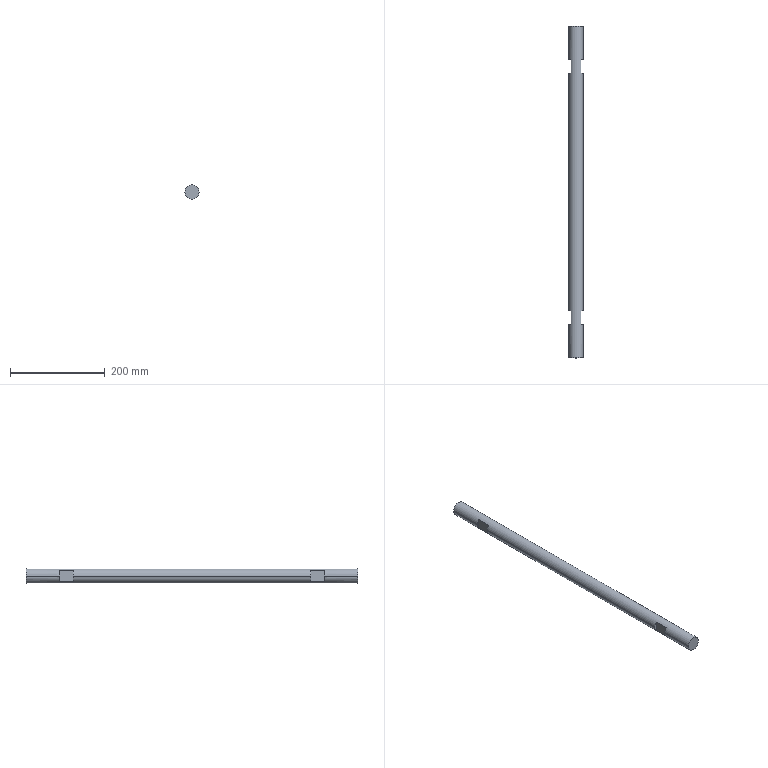Part | NX | features BREP 1 | 1 solid | 16 faces | box 30 x 700 x 30 mm | volume 485508 mm3 | plane 14 | cylinder 2 | commonest cylinder face diameters 30 x2
STEP:
#1=CARTESIAN_POINT('',(15.,-350.,0.));
#2=VERTEX_POINT('',#1);
#3=CARTESIAN_POINT('',(-15.,-350.,0.));
#4=VERTEX_POINT('',#3);
#5=CARTESIAN_POINT('',(0.,-350.,0.));
#6=DIRECTION('',(0.,-1.,0.));
#7=DIRECTION('',(1.,0.,0.));
#8=AXIS2_PLACEMENT_3D('',#5,#6,#7);
#9=CIRCLE('',#8,15.);
#10=EDGE_CURVE('',#2,#4,#9,.T.);
#11=ORIENTED_EDGE('',*,*,#10,.T.);
#12=CARTESIAN_POINT('',(0.,-350.,0.));
#13=DIRECTION('',(0.,-1.,0.));
#14=DIRECTION('',(-1.,0.,0.));
#15=AXIS2_PLACEMENT_3D('',#12,#13,#14);
#16=CIRCLE('',#15,15.);
#17=EDGE_CURVE('',#4,#2,#16,.T.);
#18=ORIENTED_EDGE('',*,*,#17,.T.);
#19=EDGE_LOOP('',(#11,#18));
#20=FACE_BOUND('',#19,.T.);
#21=CARTESIAN_POINT('',(0.,-350.,0.));
#22=DIRECTION('',(0.,1.,0.));
#23=DIRECTION('',(1.,0.,0.));
#24=AXIS2_PLACEMENT_3D('',#21,#22,#23);
#25=PLANE('',#24);
#26=ADVANCED_FACE('',(#20),#25,.F.);
#27=CARTESIAN_POINT('',(10.,-250.,-11.18));
#28=VERTEX_POINT('',#27);
#29=CARTESIAN_POINT('',(15.,-250.,0.));
#30=VERTEX_POINT('',#29);
#31=CARTESIAN_POINT('',(0.,-250.,0.));
#32=DIRECTION('',(0.,-1.,0.));
#33=DIRECTION('',(0.6667,0.,-0.7454));
#34=AXIS2_PLACEMENT_3D('',#31,#32,#33);
#35=CIRCLE('',#34,15.);
#36=EDGE_CURVE('',#28,#30,#35,.T.);
#37=ORIENTED_EDGE('',*,*,#36,.F.);
#38=CARTESIAN_POINT('',(10.,-280.,-11.18));
#39=VERTEX_POINT('',#38);
#40=CARTESIAN_POINT('',(10.,-250.,-11.18));
#41=DIRECTION('',(0.,-1.,0.));
#42=VECTOR('',#41,1000.);
#43=LINE('',#40,#42);
#44=EDGE_CURVE('',#28,#39,#43,.T.);
#45=ORIENTED_EDGE('',*,*,#44,.T.);
#46=CARTESIAN_POINT('',(15.,-280.,0.));
#47=VERTEX_POINT('',#46);
#48=CARTESIAN_POINT('',(0.,-280.,0.));
#49=DIRECTION('',(0.,1.,0.));
#50=DIRECTION('',(1.,0.,0.));
#51=AXIS2_PLACEMENT_3D('',#48,#49,#50);
#52=CIRCLE('',#51,15.);
#53=EDGE_CURVE('',#47,#39,#52,.T.);
#54=ORIENTED_EDGE('',*,*,#53,.F.);
#55=CARTESIAN_POINT('',(15.,-280.,0.));
#56=DIRECTION('',(0.,-1.,0.));
#57=VECTOR('',#56,1000.);
#58=LINE('',#55,#57);
#59=EDGE_CURVE('',#47,#2,#58,.T.);
#60=ORIENTED_EDGE('',*,*,#59,.T.);
#61=ORIENTED_EDGE('',*,*,#17,.F.);
#62=CARTESIAN_POINT('',(-15.,-280.,0.));
#63=VERTEX_POINT('',#62);
#64=CARTESIAN_POINT('',(-15.,-280.,0.));
#65=DIRECTION('',(0.,-1.,0.));
#66=VECTOR('',#65,1000.);
#67=LINE('',#64,#66);
#68=EDGE_CURVE('',#63,#4,#67,.T.);
#69=ORIENTED_EDGE('',*,*,#68,.F.);
#70=CARTESIAN_POINT('',(-10.,-280.,-11.18));
#71=VERTEX_POINT('',#70);
#72=CARTESIAN_POINT('',(0.,-280.,0.));
#73=DIRECTION('',(0.,1.,0.));
#74=DIRECTION('',(-0.6667,0.,-0.7454));
#75=AXIS2_PLACEMENT_3D('',#72,#73,#74);
#76=CIRCLE('',#75,15.);
#77=EDGE_CURVE('',#71,#63,#76,.T.);
#78=ORIENTED_EDGE('',*,*,#77,.F.);
#79=CARTESIAN_POINT('',(-10.,-250.,-11.18));
#80=VERTEX_POINT('',#79);
#81=CARTESIAN_POINT('',(-10.,-280.,-11.18));
#82=DIRECTION('',(0.,1.,0.));
#83=VECTOR('',#82,1000.);
#84=LINE('',#81,#83);
#85=EDGE_CURVE('',#71,#80,#84,.T.);
#86=ORIENTED_EDGE('',*,*,#85,.T.);
#87=CARTESIAN_POINT('',(-15.,-250.,0.));
#88=VERTEX_POINT('',#87);
#89=CARTESIAN_POINT('',(0.,-250.,0.));
#90=DIRECTION('',(0.,-1.,0.));
#91=DIRECTION('',(-1.,0.,0.));
#92=AXIS2_PLACEMENT_3D('',#89,#90,#91);
#93=CIRCLE('',#92,15.);
#94=EDGE_CURVE('',#88,#80,#93,.T.);
#95=ORIENTED_EDGE('',*,*,#94,.F.);
#96=CARTESIAN_POINT('',(-15.,250.,0.));
#97=VERTEX_POINT('',#96);
#98=CARTESIAN_POINT('',(-15.,250.,0.));
#99=DIRECTION('',(0.,-1.,0.));
#100=VECTOR('',#99,1000.);
#101=LINE('',#98,#100);
#102=EDGE_CURVE('',#97,#88,#101,.T.);
#103=ORIENTED_EDGE('',*,*,#102,.F.);
#104=CARTESIAN_POINT('',(-10.,250.,-11.18));
#105=VERTEX_POINT('',#104);
#106=CARTESIAN_POINT('',(0.,250.,0.));
#107=DIRECTION('',(0.,1.,0.));
#108=DIRECTION('',(-0.6667,0.,-0.7454));
#109=AXIS2_PLACEMENT_3D('',#106,#107,#108);
#110=CIRCLE('',#109,15.);
#111=EDGE_CURVE('',#105,#97,#110,.T.);
#112=ORIENTED_EDGE('',*,*,#111,.F.);
#113=CARTESIAN_POINT('',(-10.,280.,-11.18));
#114=VERTEX_POINT('',#113);
#115=CARTESIAN_POINT('',(-10.,250.,-11.18));
#116=DIRECTION('',(0.,1.,0.));
#117=VECTOR('',#116,1000.);
#118=LINE('',#115,#117);
#119=EDGE_CURVE('',#105,#114,#118,.T.);
#120=ORIENTED_EDGE('',*,*,#119,.T.);
#121=CARTESIAN_POINT('',(-15.,280.,0.));
#122=VERTEX_POINT('',#121);
#123=CARTESIAN_POINT('',(0.,280.,0.));
#124=DIRECTION('',(0.,-1.,0.));
#125=DIRECTION('',(-1.,0.,0.));
#126=AXIS2_PLACEMENT_3D('',#123,#124,#125);
#127=CIRCLE('',#126,15.);
#128=EDGE_CURVE('',#122,#114,#127,.T.);
#129=ORIENTED_EDGE('',*,*,#128,.F.);
#130=CARTESIAN_POINT('',(-15.,350.,0.));
#131=VERTEX_POINT('',#130);
#132=CARTESIAN_POINT('',(-15.,350.,0.));
#133=DIRECTION('',(0.,-1.,0.));
#134=VECTOR('',#133,1000.);
#135=LINE('',#132,#134);
#136=EDGE_CURVE('',#122,#131,#135,.F.);
#137=ORIENTED_EDGE('',*,*,#136,.T.);
#138=CARTESIAN_POINT('',(15.,350.,0.));
#139=VERTEX_POINT('',#138);
#140=CARTESIAN_POINT('',(0.,350.,0.));
#141=DIRECTION('',(0.,1.,0.));
#142=DIRECTION('',(1.,0.,0.));
#143=AXIS2_PLACEMENT_3D('',#140,#141,#142);
#144=CIRCLE('',#143,15.);
#145=EDGE_CURVE('',#139,#131,#144,.T.);
#146=ORIENTED_EDGE('',*,*,#145,.F.);
#147=CARTESIAN_POINT('',(15.,280.,0.));
#148=VERTEX_POINT('',#147);
#149=CARTESIAN_POINT('',(15.,350.,0.));
#150=DIRECTION('',(0.,-1.,0.));
#151=VECTOR('',#150,1000.);
#152=LINE('',#149,#151);
#153=EDGE_CURVE('',#148,#139,#152,.F.);
#154=ORIENTED_EDGE('',*,*,#153,.F.);
#155=CARTESIAN_POINT('',(10.,280.,-11.18));
#156=VERTEX_POINT('',#155);
#157=CARTESIAN_POINT('',(0.,280.,0.));
#158=DIRECTION('',(0.,-1.,0.));
#159=DIRECTION('',(0.6667,0.,-0.7454));
#160=AXIS2_PLACEMENT_3D('',#157,#158,#159);
#161=CIRCLE('',#160,15.);
#162=EDGE_CURVE('',#156,#148,#161,.T.);
#163=ORIENTED_EDGE('',*,*,#162,.F.);
#164=CARTESIAN_POINT('',(10.,250.,-11.18));
#165=VERTEX_POINT('',#164);
#166=CARTESIAN_POINT('',(10.,280.,-11.18));
#167=DIRECTION('',(0.,-1.,0.));
#168=VECTOR('',#167,1000.);
#169=LINE('',#166,#168);
#170=EDGE_CURVE('',#156,#165,#169,.T.);
#171=ORIENTED_EDGE('',*,*,#170,.T.);
#172=CARTESIAN_POINT('',(15.,250.,0.));
#173=VERTEX_POINT('',#172);
#174=CARTESIAN_POINT('',(0.,250.,0.));
#175=DIRECTION('',(0.,1.,0.));
#176=DIRECTION('',(1.,0.,0.));
#177=AXIS2_PLACEMENT_3D('',#174,#175,#176);
#178=CIRCLE('',#177,15.);
#179=EDGE_CURVE('',#173,#165,#178,.T.);
#180=ORIENTED_EDGE('',*,*,#179,.F.);
#181=CARTESIAN_POINT('',(15.,250.,0.));
#182=DIRECTION('',(0.,-1.,0.));
#183=VECTOR('',#182,1000.);
#184=LINE('',#181,#183);
#185=EDGE_CURVE('',#173,#30,#184,.T.);
#186=ORIENTED_EDGE('',*,*,#185,.T.);
#187=EDGE_LOOP('',(#37,#45,#54,#60,#61,#69,#78,#86,#95,#103,#112,#120,#129,#137,#146,#154,#163,#171,#180,#186));
#188=FACE_BOUND('',#187,.T.);
#189=CARTESIAN_POINT('',(0.,0.,0.));
#190=DIRECTION('',(0.,1.,0.));
#191=DIRECTION('',(-1.,0.,0.));
#192=AXIS2_PLACEMENT_3D('',#189,#190,#191);
#193=CYLINDRICAL_SURFACE('',#192,15.);
#194=ADVANCED_FACE('',(#188),#193,.T.);
#195=CARTESIAN_POINT('',(-10.,-250.,11.18));
#196=VERTEX_POINT('',#195);
#197=CARTESIAN_POINT('',(0.,-250.,0.));
#198=DIRECTION('',(0.,-1.,0.));
#199=DIRECTION('',(-0.6667,0.,0.7454));
#200=AXIS2_PLACEMENT_3D('',#197,#198,#199);
#201=CIRCLE('',#200,15.);
#202=EDGE_CURVE('',#196,#88,#201,.T.);
#203=ORIENTED_EDGE('',*,*,#202,.F.);
#204=CARTESIAN_POINT('',(-10.,-280.,11.18));
#205=VERTEX_POINT('',#204);
#206=CARTESIAN_POINT('',(-10.,-250.,11.18));
#207=DIRECTION('',(0.,-1.,0.));
#208=VECTOR('',#207,1000.);
#209=LINE('',#206,#208);
#210=EDGE_CURVE('',#196,#205,#209,.T.);
#211=ORIENTED_EDGE('',*,*,#210,.T.);
#212=CARTESIAN_POINT('',(0.,-280.,0.));
#213=DIRECTION('',(0.,1.,0.));
#214=DIRECTION('',(-1.,0.,0.));
#215=AXIS2_PLACEMENT_3D('',#212,#213,#214);
#216=CIRCLE('',#215,15.);
#217=EDGE_CURVE('',#63,#205,#216,.T.);
#218=ORIENTED_EDGE('',*,*,#217,.F.);
#219=ORIENTED_EDGE('',*,*,#68,.T.);
#220=ORIENTED_EDGE('',*,*,#10,.F.);
#221=ORIENTED_EDGE('',*,*,#59,.F.);
#222=CARTESIAN_POINT('',(10.,-280.,11.18));
#223=VERTEX_POINT('',#222);
#224=CARTESIAN_POINT('',(0.,-280.,0.));
#225=DIRECTION('',(0.,1.,0.));
#226=DIRECTION('',(0.6667,0.,0.7454));
#227=AXIS2_PLACEMENT_3D('',#224,#225,#226);
#228=CIRCLE('',#227,15.);
#229=EDGE_CURVE('',#223,#47,#228,.T.);
#230=ORIENTED_EDGE('',*,*,#229,.F.);
#231=CARTESIAN_POINT('',(10.,-250.,11.18));
#232=VERTEX_POINT('',#231);
#233=CARTESIAN_POINT('',(10.,-280.,11.18));
#234=DIRECTION('',(0.,1.,0.));
#235=VECTOR('',#234,1000.);
#236=LINE('',#233,#235);
#237=EDGE_CURVE('',#223,#232,#236,.T.);
#238=ORIENTED_EDGE('',*,*,#237,.T.);
#239=CARTESIAN_POINT('',(0.,-250.,0.));
#240=DIRECTION('',(0.,-1.,0.));
#241=DIRECTION('',(1.,0.,0.));
#242=AXIS2_PLACEMENT_3D('',#239,#240,#241);
#243=CIRCLE('',#242,15.);
#244=EDGE_CURVE('',#30,#232,#243,.T.);
#245=ORIENTED_EDGE('',*,*,#244,.F.);
#246=ORIENTED_EDGE('',*,*,#185,.F.);
#247=CARTESIAN_POINT('',(10.,250.,11.18));
#248=VERTEX_POINT('',#247);
#249=CARTESIAN_POINT('',(0.,250.,0.));
#250=DIRECTION('',(0.,1.,0.));
#251=DIRECTION('',(0.6667,0.,0.7454));
#252=AXIS2_PLACEMENT_3D('',#249,#250,#251);
#253=CIRCLE('',#252,15.);
#254=EDGE_CURVE('',#248,#173,#253,.T.);
#255=ORIENTED_EDGE('',*,*,#254,.F.);
#256=CARTESIAN_POINT('',(10.,280.,11.18));
#257=VERTEX_POINT('',#256);
#258=CARTESIAN_POINT('',(10.,250.,11.18));
#259=DIRECTION('',(0.,1.,0.));
#260=VECTOR('',#259,1000.);
#261=LINE('',#258,#260);
#262=EDGE_CURVE('',#248,#257,#261,.T.);
#263=ORIENTED_EDGE('',*,*,#262,.T.);
#264=CARTESIAN_POINT('',(0.,280.,0.));
#265=DIRECTION('',(0.,-1.,0.));
#266=DIRECTION('',(1.,0.,0.));
#267=AXIS2_PLACEMENT_3D('',#264,#265,#266);
#268=CIRCLE('',#267,15.);
#269=EDGE_CURVE('',#148,#257,#268,.T.);
#270=ORIENTED_EDGE('',*,*,#269,.F.);
#271=ORIENTED_EDGE('',*,*,#153,.T.);
#272=CARTESIAN_POINT('',(0.,350.,0.));
#273=DIRECTION('',(0.,1.,0.));
#274=DIRECTION('',(-1.,0.,0.));
#275=AXIS2_PLACEMENT_3D('',#272,#273,#274);
#276=CIRCLE('',#275,15.);
#277=EDGE_CURVE('',#131,#139,#276,.T.);
#278=ORIENTED_EDGE('',*,*,#277,.F.);
#279=ORIENTED_EDGE('',*,*,#136,.F.);
#280=CARTESIAN_POINT('',(-10.,280.,11.18));
#281=VERTEX_POINT('',#280);
#282=CARTESIAN_POINT('',(0.,280.,0.));
#283=DIRECTION('',(0.,-1.,0.));
#284=DIRECTION('',(-0.6667,0.,0.7454));
#285=AXIS2_PLACEMENT_3D('',#282,#283,#284);
#286=CIRCLE('',#285,15.);
#287=EDGE_CURVE('',#281,#122,#286,.T.);
#288=ORIENTED_EDGE('',*,*,#287,.F.);
#289=CARTESIAN_POINT('',(-10.,250.,11.18));
#290=VERTEX_POINT('',#289);
#291=CARTESIAN_POINT('',(-10.,280.,11.18));
#292=DIRECTION('',(0.,-1.,0.));
#293=VECTOR('',#292,1000.);
#294=LINE('',#291,#293);
#295=EDGE_CURVE('',#281,#290,#294,.T.);
#296=ORIENTED_EDGE('',*,*,#295,.T.);
#297=CARTESIAN_POINT('',(0.,250.,0.));
#298=DIRECTION('',(0.,1.,0.));
#299=DIRECTION('',(-1.,0.,0.));
#300=AXIS2_PLACEMENT_3D('',#297,#298,#299);
#301=CIRCLE('',#300,15.);
#302=EDGE_CURVE('',#97,#290,#301,.T.);
#303=ORIENTED_EDGE('',*,*,#302,.F.);
#304=ORIENTED_EDGE('',*,*,#102,.T.);
#305=EDGE_LOOP('',(#203,#211,#218,#219,#220,#221,#230,#238,#245,#246,#255,#263,#270,#271,#278,#279,#288,#296,#303,#304));
#306=FACE_BOUND('',#305,.T.);
#307=CARTESIAN_POINT('',(0.,0.,0.));
#308=DIRECTION('',(0.,1.,0.));
#309=DIRECTION('',(-1.,0.,0.));
#310=AXIS2_PLACEMENT_3D('',#307,#308,#309);
#311=CYLINDRICAL_SURFACE('',#310,15.);
#312=ADVANCED_FACE('',(#306),#311,.T.);
#313=ORIENTED_EDGE('',*,*,#111,.T.);
#314=ORIENTED_EDGE('',*,*,#302,.T.);
#315=CARTESIAN_POINT('',(-10.,250.,-11.18));
#316=DIRECTION('',(0.,0.,1.));
#317=VECTOR('',#316,1000.);
#318=LINE('',#315,#317);
#319=EDGE_CURVE('',#105,#290,#318,.T.);
#320=ORIENTED_EDGE('',*,*,#319,.F.);
#321=EDGE_LOOP('',(#313,#314,#320));
#322=FACE_BOUND('',#321,.T.);
#323=CARTESIAN_POINT('',(-50.874,250.,0.));
#324=DIRECTION('',(0.,1.,0.));
#325=DIRECTION('',(1.,0.,0.));
#326=AXIS2_PLACEMENT_3D('',#323,#324,#325);
#327=PLANE('',#326);
#328=ADVANCED_FACE('',(#322),#327,.T.);
#329=ORIENTED_EDGE('',*,*,#119,.F.);
#330=ORIENTED_EDGE('',*,*,#319,.T.);
#331=ORIENTED_EDGE('',*,*,#295,.F.);
#332=CARTESIAN_POINT('',(-10.,280.,-11.18));
#333=DIRECTION('',(0.,0.,1.));
#334=VECTOR('',#333,1000.);
#335=LINE('',#332,#334);
#336=EDGE_CURVE('',#114,#281,#335,.T.);
#337=ORIENTED_EDGE('',*,*,#336,.F.);
#338=EDGE_LOOP('',(#329,#330,#331,#337));
#339=FACE_BOUND('',#338,.T.);
#340=CARTESIAN_POINT('',(-10.,280.,0.));
#341=DIRECTION('',(1.,0.,0.));
#342=DIRECTION('',(0.,1.,0.));
#343=AXIS2_PLACEMENT_3D('',#340,#341,#342);
#344=PLANE('',#343);
#345=ADVANCED_FACE('',(#339),#344,.F.);
#346=ORIENTED_EDGE('',*,*,#287,.T.);
#347=ORIENTED_EDGE('',*,*,#128,.T.);
#348=ORIENTED_EDGE('',*,*,#336,.T.);
#349=EDGE_LOOP('',(#346,#347,#348));
#350=FACE_BOUND('',#349,.T.);
#351=CARTESIAN_POINT('',(-10.,280.,0.));
#352=DIRECTION('',(0.,-1.,0.));
#353=DIRECTION('',(0.,0.,-1.));
#354=AXIS2_PLACEMENT_3D('',#351,#352,#353);
#355=PLANE('',#354);
#356=ADVANCED_FACE('',(#350),#355,.T.);
#357=ORIENTED_EDGE('',*,*,#145,.T.);
#358=ORIENTED_EDGE('',*,*,#277,.T.);
#359=EDGE_LOOP('',(#357,#358));
#360=FACE_BOUND('',#359,.T.);
#361=CARTESIAN_POINT('',(0.,350.,0.));
#362=DIRECTION('',(0.,1.,0.));
#363=DIRECTION('',(1.,0.,0.));
#364=AXIS2_PLACEMENT_3D('',#361,#362,#363);
#365=PLANE('',#364);
#366=ADVANCED_FACE('',(#360),#365,.T.);
#367=ORIENTED_EDGE('',*,*,#162,.T.);
#368=ORIENTED_EDGE('',*,*,#269,.T.);
#369=CARTESIAN_POINT('',(10.,280.,-11.18));
#370=DIRECTION('',(0.,0.,1.));
#371=VECTOR('',#370,1000.);
#372=LINE('',#369,#371);
#373=EDGE_CURVE('',#156,#257,#372,.T.);
#374=ORIENTED_EDGE('',*,*,#373,.F.);
#375=EDGE_LOOP('',(#367,#368,#374));
#376=FACE_BOUND('',#375,.T.);
#377=CARTESIAN_POINT('',(-10.,280.,0.));
#378=DIRECTION('',(0.,-1.,0.));
#379=DIRECTION('',(0.,0.,-1.));
#380=AXIS2_PLACEMENT_3D('',#377,#378,#379);
#381=PLANE('',#380);
#382=ADVANCED_FACE('',(#376),#381,.T.);
#383=CARTESIAN_POINT('',(10.,250.,-11.18));
#384=DIRECTION('',(0.,0.,1.));
#385=VECTOR('',#384,1000.);
#386=LINE('',#383,#385);
#387=EDGE_CURVE('',#165,#248,#386,.T.);
#388=ORIENTED_EDGE('',*,*,#387,.F.);
#389=ORIENTED_EDGE('',*,*,#170,.F.);
#390=ORIENTED_EDGE('',*,*,#373,.T.);
#391=ORIENTED_EDGE('',*,*,#262,.F.);
#392=EDGE_LOOP('',(#388,#389,#390,#391));
#393=FACE_BOUND('',#392,.T.);
#394=CARTESIAN_POINT('',(10.,280.,0.));
#395=DIRECTION('',(1.,0.,0.));
#396=DIRECTION('',(0.,1.,0.));
#397=AXIS2_PLACEMENT_3D('',#394,#395,#396);
#398=PLANE('',#397);
#399=ADVANCED_FACE('',(#393),#398,.T.);
#400=ORIENTED_EDGE('',*,*,#254,.T.);
#401=ORIENTED_EDGE('',*,*,#179,.T.);
#402=ORIENTED_EDGE('',*,*,#387,.T.);
#403=EDGE_LOOP('',(#400,#401,#402));
#404=FACE_BOUND('',#403,.T.);
#405=CARTESIAN_POINT('',(-50.874,250.,0.));
#406=DIRECTION('',(0.,1.,0.));
#407=DIRECTION('',(1.,0.,0.));
#408=AXIS2_PLACEMENT_3D('',#405,#406,#407);
#409=PLANE('',#408);
#410=ADVANCED_FACE('',(#404),#409,.T.);
#411=ORIENTED_EDGE('',*,*,#36,.T.);
#412=ORIENTED_EDGE('',*,*,#244,.T.);
#413=CARTESIAN_POINT('',(10.,-250.,-11.18));
#414=DIRECTION('',(0.,0.,1.));
#415=VECTOR('',#414,1000.);
#416=LINE('',#413,#415);
#417=EDGE_CURVE('',#28,#232,#416,.T.);
#418=ORIENTED_EDGE('',*,*,#417,.F.);
#419=EDGE_LOOP('',(#411,#412,#418));
#420=FACE_BOUND('',#419,.T.);
#421=CARTESIAN_POINT('',(50.874,-250.,0.));
#422=DIRECTION('',(0.,-1.,0.));
#423=DIRECTION('',(0.,0.,-1.));
#424=AXIS2_PLACEMENT_3D('',#421,#422,#423);
#425=PLANE('',#424);
#426=ADVANCED_FACE('',(#420),#425,.T.);
#427=CARTESIAN_POINT('',(10.,-280.,-11.18));
#428=DIRECTION('',(0.,0.,1.));
#429=VECTOR('',#428,1000.);
#430=LINE('',#427,#429);
#431=EDGE_CURVE('',#39,#223,#430,.T.);
#432=ORIENTED_EDGE('',*,*,#431,.F.);
#433=ORIENTED_EDGE('',*,*,#44,.F.);
#434=ORIENTED_EDGE('',*,*,#417,.T.);
#435=ORIENTED_EDGE('',*,*,#237,.F.);
#436=EDGE_LOOP('',(#432,#433,#434,#435));
#437=FACE_BOUND('',#436,.T.);
#438=CARTESIAN_POINT('',(10.,280.,0.));
#439=DIRECTION('',(1.,0.,0.));
#440=DIRECTION('',(0.,1.,0.));
#441=AXIS2_PLACEMENT_3D('',#438,#439,#440);
#442=PLANE('',#441);
#443=ADVANCED_FACE('',(#437),#442,.T.);
#444=ORIENTED_EDGE('',*,*,#229,.T.);
#445=ORIENTED_EDGE('',*,*,#53,.T.);
#446=ORIENTED_EDGE('',*,*,#431,.T.);
#447=EDGE_LOOP('',(#444,#445,#446));
#448=FACE_BOUND('',#447,.T.);
#449=CARTESIAN_POINT('',(10.,-280.,0.));
#450=DIRECTION('',(0.,1.,0.));
#451=DIRECTION('',(1.,0.,0.));
#452=AXIS2_PLACEMENT_3D('',#449,#450,#451);
#453=PLANE('',#452);
#454=ADVANCED_FACE('',(#448),#453,.T.);
#455=ORIENTED_EDGE('',*,*,#77,.T.);
#456=ORIENTED_EDGE('',*,*,#217,.T.);
#457=CARTESIAN_POINT('',(-10.,-280.,-11.18));
#458=DIRECTION('',(0.,0.,1.));
#459=VECTOR('',#458,1000.);
#460=LINE('',#457,#459);
#461=EDGE_CURVE('',#71,#205,#460,.T.);
#462=ORIENTED_EDGE('',*,*,#461,.F.);
#463=EDGE_LOOP('',(#455,#456,#462));
#464=FACE_BOUND('',#463,.T.);
#465=CARTESIAN_POINT('',(10.,-280.,0.));
#466=DIRECTION('',(0.,1.,0.));
#467=DIRECTION('',(1.,0.,0.));
#468=AXIS2_PLACEMENT_3D('',#465,#466,#467);
#469=PLANE('',#468);
#470=ADVANCED_FACE('',(#464),#469,.T.);
#471=ORIENTED_EDGE('',*,*,#85,.F.);
#472=ORIENTED_EDGE('',*,*,#461,.T.);
#473=ORIENTED_EDGE('',*,*,#210,.F.);
#474=CARTESIAN_POINT('',(-10.,-250.,-11.18));
#475=DIRECTION('',(0.,0.,1.));
#476=VECTOR('',#475,1000.);
#477=LINE('',#474,#476);
#478=EDGE_CURVE('',#80,#196,#477,.T.);
#479=ORIENTED_EDGE('',*,*,#478,.F.);
#480=EDGE_LOOP('',(#471,#472,#473,#479));
#481=FACE_BOUND('',#480,.T.);
#482=CARTESIAN_POINT('',(-10.,280.,0.));
#483=DIRECTION('',(1.,0.,0.));
#484=DIRECTION('',(0.,1.,0.));
#485=AXIS2_PLACEMENT_3D('',#482,#483,#484);
#486=PLANE('',#485);
#487=ADVANCED_FACE('',(#481),#486,.F.);
#488=ORIENTED_EDGE('',*,*,#202,.T.);
#489=ORIENTED_EDGE('',*,*,#94,.T.);
#490=ORIENTED_EDGE('',*,*,#478,.T.);
#491=EDGE_LOOP('',(#488,#489,#490));
#492=FACE_BOUND('',#491,.T.);
#493=CARTESIAN_POINT('',(50.874,-250.,0.));
#494=DIRECTION('',(0.,-1.,0.));
#495=DIRECTION('',(0.,0.,-1.));
#496=AXIS2_PLACEMENT_3D('',#493,#494,#495);
#497=PLANE('',#496);
#498=ADVANCED_FACE('',(#492),#497,.T.);
#499=CLOSED_SHELL('',(#26,#194,#312,#328,#345,#356,#366,#382,#399,#410,#426,#443,#454,#470,#487,#498));
#500=MANIFOLD_SOLID_BREP('',#499);
#501=(LENGTH_UNIT()NAMED_UNIT(*)SI_UNIT(.MILLI.,.METRE.));
#502=UNCERTAINTY_MEASURE_WITH_UNIT(LENGTH_MEASURE(0.00001),#501,'','');
#503=(NAMED_UNIT(*)PLANE_ANGLE_UNIT()SI_UNIT($,.RADIAN.));
#504=(NAMED_UNIT(*)SI_UNIT($,.STERADIAN.)SOLID_ANGLE_UNIT());
#505=(GEOMETRIC_REPRESENTATION_CONTEXT(3)GLOBAL_UNCERTAINTY_ASSIGNED_CONTEXT((#502))GLOBAL_UNIT_ASSIGNED_CONTEXT((#501,#503,#504))REPRESENTATION_CONTEXT('',''));
#506=ADVANCED_BREP_SHAPE_REPRESENTATION('',(#500),#505);